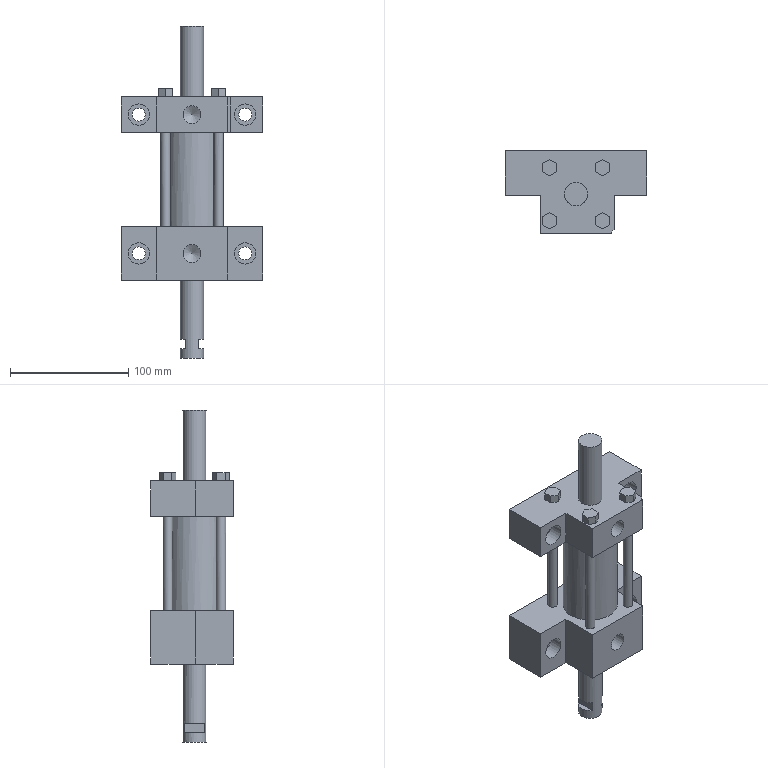Part | STEP file | solid 171 | 1 solid | 81 faces | box 120 x 70 x 281 mm | volume 651567 mm3 | plane 62 | cylinder 17 | cone 2 | commonest cylinder face diameters 8 x4 11 x4 18 x4 15 x2 20 x2 46 x1